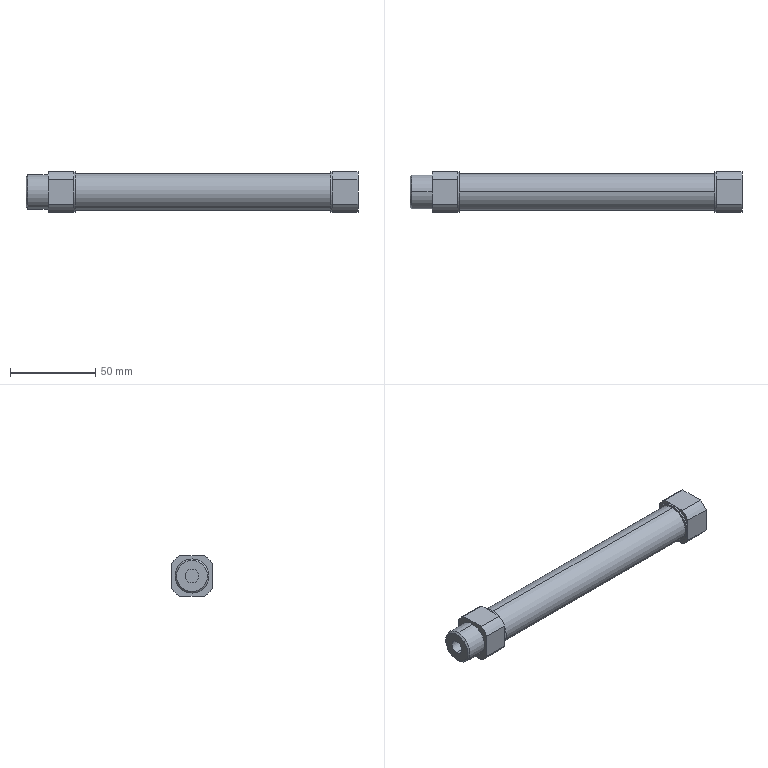Part | SolidWorks | CDM2BZ20x120-D_1.stp | 1 solid | 60 faces | box 195 x 24 x 24 mm | volume 39099 mm3 | plane 28 | cylinder 26 | cone 6 | commonest cylinder face diameters 28 x8 8 x4 8.566 x4 24 x4 18 x2 20 x2